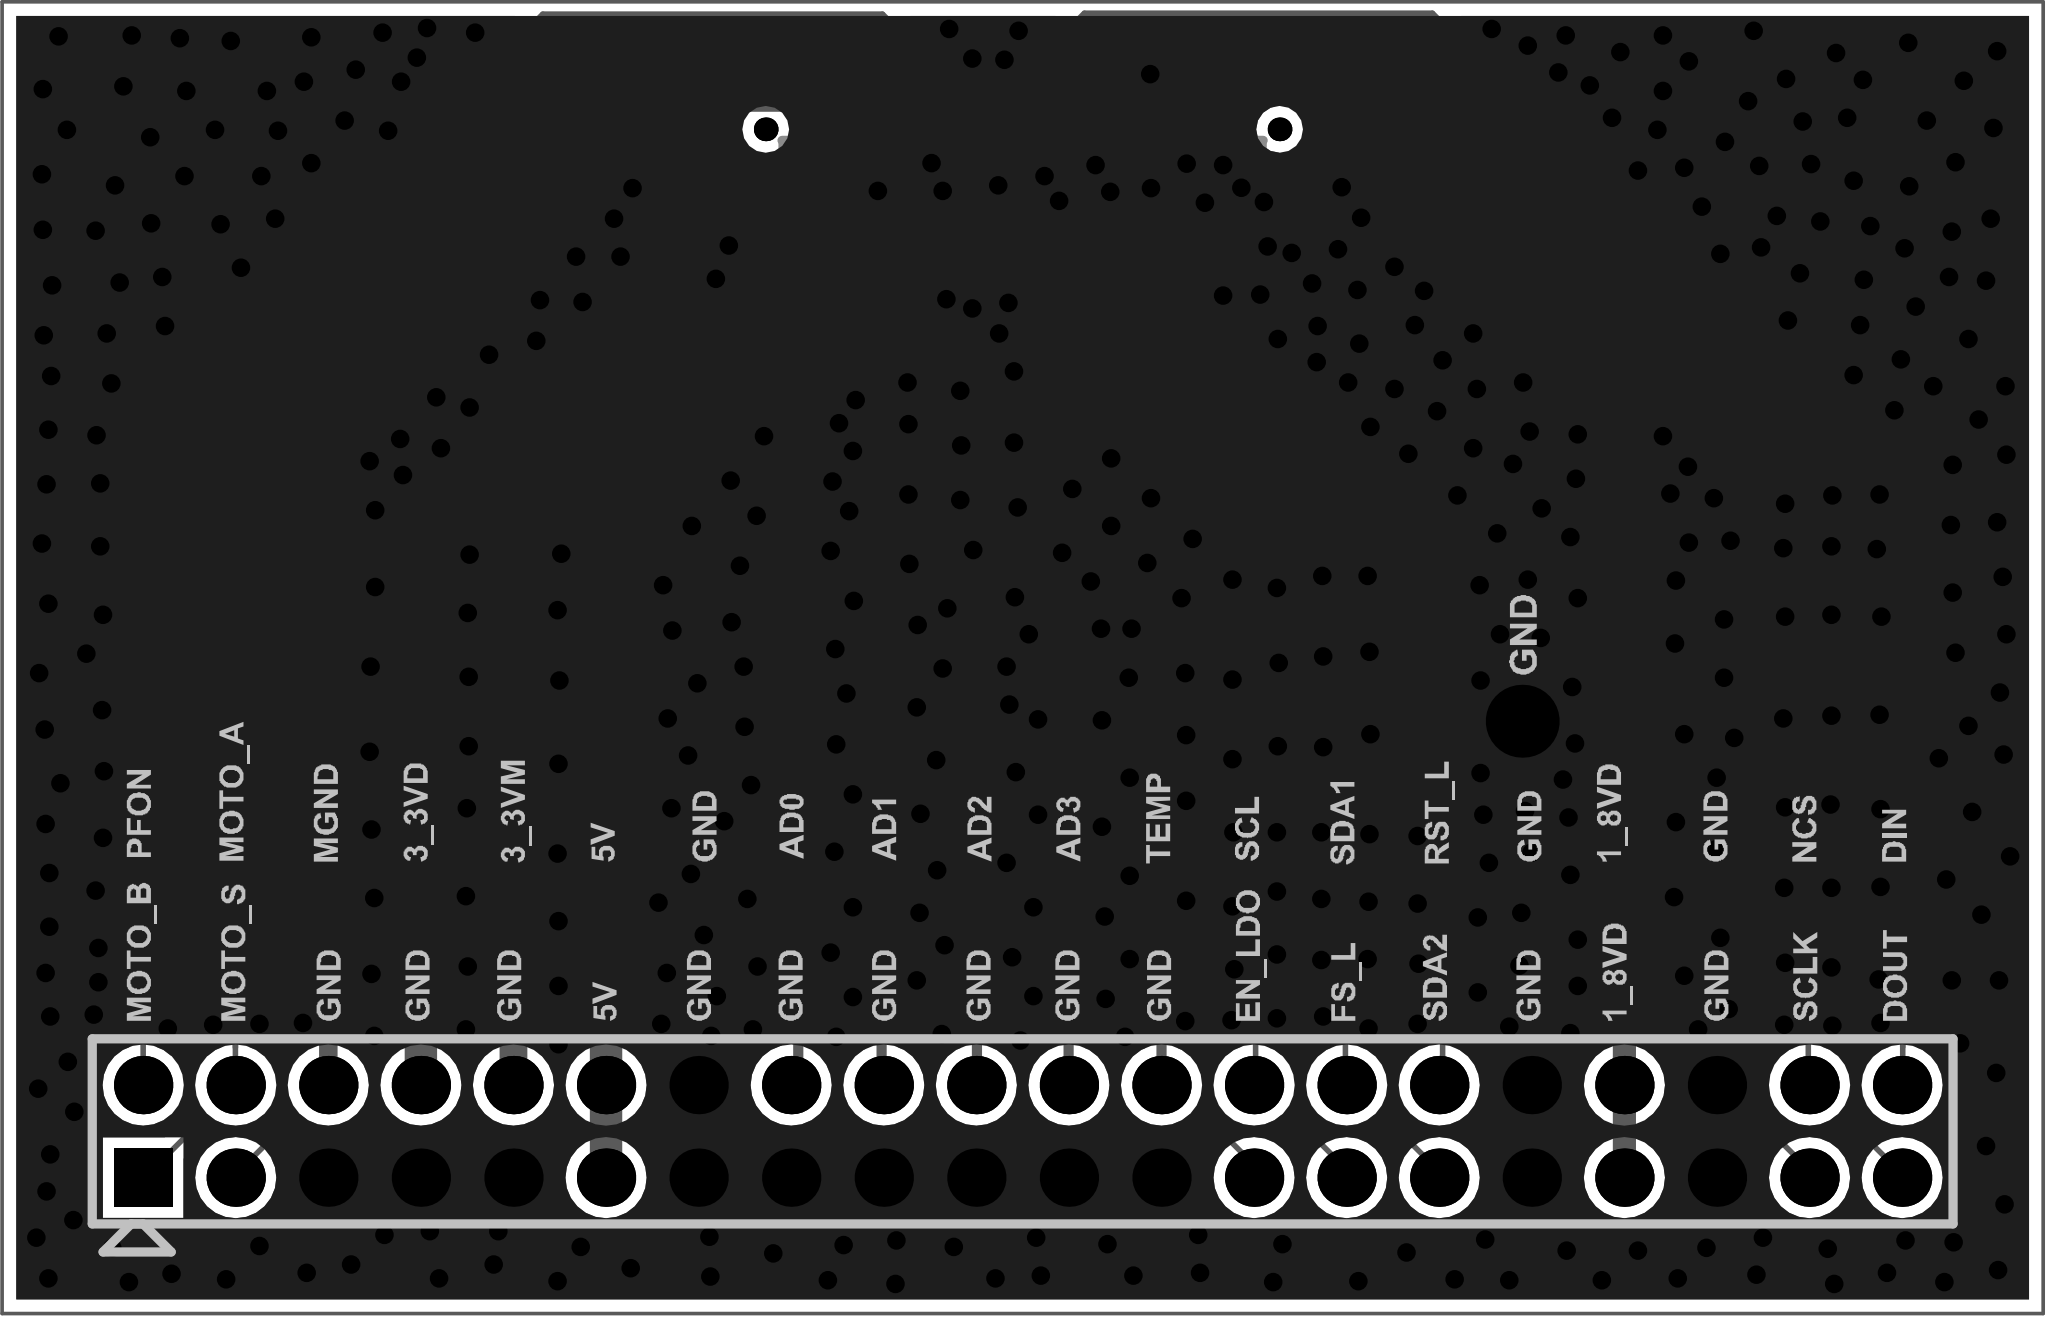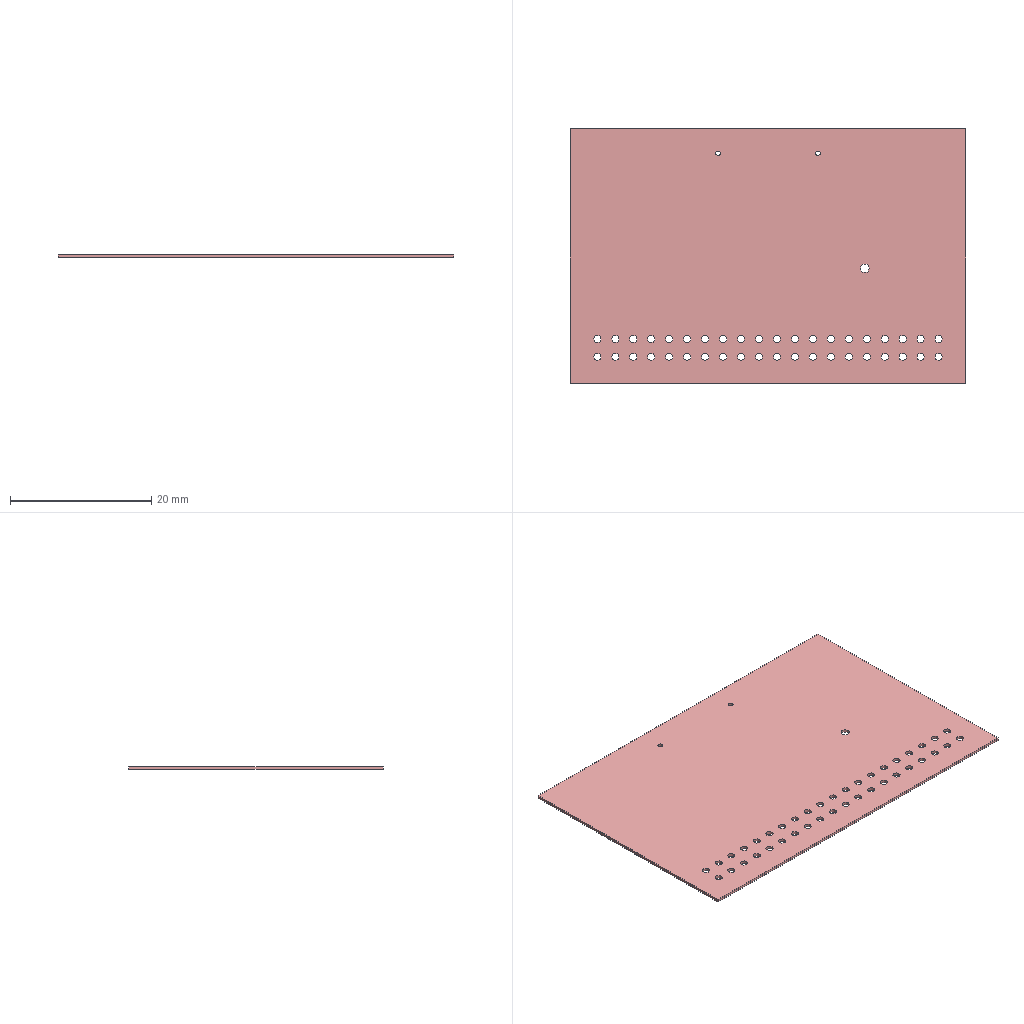Circuit board layout | Altium Designer | box 56 x 36 x 0.4 mm
Layer stack:
# Altium Designer layer stack of  (unit mm; dielectric type: 0 none, 1 core, 2 prepreg, 3 surface material)
index,name,kind,layer,copper_thickness_mm,dielectric_type,dielectric_thickness_mm,dielectric_material,dielectric_constant
0,Top Paste,other,,,,,,
1,Top Overlay,other,,,,,,
2,Top Solder,dielectric,,,3,0.0102,Solder Resist,3.5
3,Top Layer,copper,Top Layer,0.0356,,,,
4,Dielectric1,dielectric,,,0,0.32,FR-4,4.8
5,Bottom Layer,copper,Bottom Layer,0.0356,,,,
6,Bottom Solder,dielectric,,,3,0.0102,Solder Resist,3.5
7,Bottom Overlay,other,,,,,,
8,Bottom Paste,other,,,,,,
# drill layer pairs: low layer,high layer
drill_pair,Top Layer,Bottom Layer
Part placement:
Designator,Comment,Layer,Footprint,Center-X(mm),Center-Y(mm),Rotation
P2,#NAME?,TopLayer,HDR-TH_40P-P2.54-V-F-R2-C20-S2.54,28,5,360
P1,#NAME?,BottomLayer,CONN-SMD_DF12A-3.0-50DS-0.5,28,31,180
Pad and via stacks:
# Altium Designer via and pad stacks of  (unit mm). Each distinct definition once, with the count of objects using it.
# via: kind,start_layer,end_layer,hole_mm,diameter_mm,mode(0 simple;1 top-mid-bottom;2 full stack),diameter_per_layer,count,example_net
# pad: kind,layer,hole_mm,hole_type(0 round;1 square;2 slot),plating,top_size,top_shape(1 round;2 rect;3 octagon;9 rounded rect),mid_size,bottom_size,mode,footprint,size_per_layer,count,example
pad,Multi-Layer,1,0,plated,1.6x1.6,1,1.6x1.6,1.6x1.6,0,HDR-TH_40P-P2.54-V-F-R2-C20-S2.54,,39,P2.40
pad,Multi-Layer,1,0,plated,1.6x1.6,2,1.6x1.6,1.6x1.6,0,HDR-TH_40P-P2.54-V-F-R2-C20-S2.54,,1,P2.1
pad,Multi-Layer,1.2,0,plated,2x2,1,2x2,2x2,0,,,1,0
pad,Multi-Layer,0.65,0,unplated,0.65x0.65,1,0.65x0.65,0.65x0.65,0,CONN-SMD_DF12A-3.0-50DS-0.5,,2,P1.0
pad,Bottom Layer,0,0,plated,0.2972x1.598,2,0.2972x1.598,0.2972x1.598,0,CONN-SMD_DF12A-3.0-50DS-0.5,,50,P1.50
pad,Bottom Layer,0,0,plated,0.7976x1.796,2,0.7976x1.796,0.7976x1.796,0,CONN-SMD_DF12A-3.0-50DS-0.5,,2,P1.52
via,Top Layer,Bottom Layer,0.3048,0.508,0,,502,GND
Copper pours:
name,layer,net,type(0 solid;1 hatched;2 none)
Bottom Layer-No Net,Bottom Layer,GND,0
Bottom Layer-No Net,Top Layer,GND,0
Design rules, without the lines most boards share:
# Altium Designer design rules of  (exported by Altium Designer, unit mm)
# columns: name | kind | enabled | priority | scope1 | scope2 | descriptor | typed fields (field=value)
Clearance_1 | 0 | enabled | 1 | inpolygon | All | Clearance Constraint (Gap=12mil) (inpolygon),(All) | gap=0.3048
Clearance | 0 | enabled | 2 | All | All | Clearance Constraint (Gap=6mil) (All),(All) | gap=0.1524
PlaneConnect | 6 | enabled | 1 | All | All | Power Plane Connect Rule(Direct Connect )(Expansion=20mil) (Conductor Width=10mil) (Air Gap=10mil) (Entries=4) (All) | relief_conductor_width=0.254 relief_entries=4 relief_expansion=0.508
PlaneClearance | 12 | enabled | 1 | All | All | Power Plane Clearance (Clearance =6mil) (All) | clearance=0.1524
PolygonConnect | 20 | enabled | 1 | All | All | Polygon Connect Rule(Direct Connect )(Conductor Width=10mil) (Relief Angle=90 Angle) (Entries=4) (Air Gap Width=10mil) (All),(All) | connect_style(0=relief,1=direct,2=none)=1 relief_conductor_width=0.254 relief_entries=4
Width | 2 | enabled | 1 | All | All | Width Constraint (Min=6mil) (Max=80mil) (Preferred=6mil) (All) |
RoutingVias | 11 | enabled | 1 | All | All | Routing Via (MinHoleWidth=12mil) (MaxHoleWidth=12mil) (PreferredHoleWidth=12mil) (MinWidth=20mil) (MaxWidth=20mil) (PreferedWidth=20mil) (All) | via_min_hole=0.3048 via_max_hole=0.3048 via_preferred_diameter=0.508 via_preferred_hole=0.3048
PasteMaskExpansion | 14 | enabled | 1 | All | All | Paste Mask Expansion (Expansion =0mil) (All) | expansion=0
SolderMaskExpansion | 13 | enabled | 1 | All | All | Solder Mask Expansion (Expansion =4mil) (All) | expansion=0.1016
HoleSize | 42 | enabled | 1 | All | All | Hole Size Constraint (Min=1mil) (Max=500mil) (All) |
DiffPairsRouting | 51 | enabled | 1 | All | All | Differential Pairs Uncoupled Length using the Gap Constraints (Min=6mil) (Max=6mil) (Prefered=6mil)  and Width Constraints (Min=15mil) (Max=15mil) (Prefered=15mil) (All) |
HoleToHoleClearance | 52 | enabled | 1 | All | All | Hole To Hole Clearance (Gap=0mil) (All),(All) | gap=0
MinimumSolderMaskSliver | 53 | enabled | 1 | All | All | Minimum Solder Mask Sliver (Gap=0mil) (All),(All) |
SilkscreenOverComponentPads | 54 | enabled | 1 | IsPad | All | Silk To Solder Mask (Clearance=0mil) (IsPad),(All) |
SilkToSilkClearance | 55 | enabled | 1 | All | All | Silk to Silk (Clearance=0mil) (All),(All) |
Classes set for this board:
# Altium Designer classes of  (member kind: 0 net, 1 component, 2 from-to, 3 pad, 4 layer, 5 differential pair, 6 design channel, 7 polygon, 8 structure, 9 xSignal)
# columns: class name | member kind | superclass | members
1_P1.schdoc | 1 | no | P1; P2; P1;